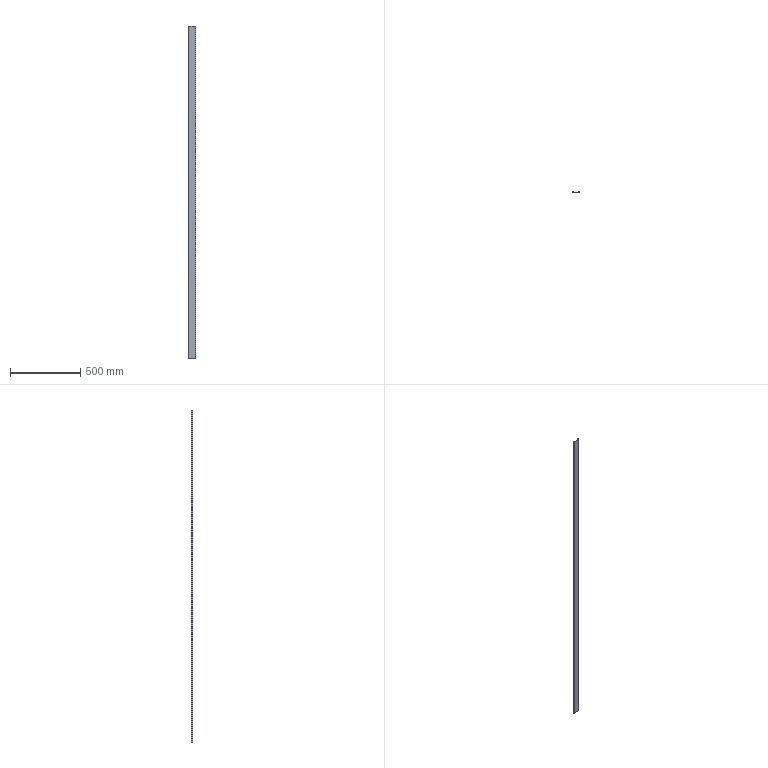Part | STEP file | 31E-01026QY25 | 1 solid | 32 faces | box 50 x 9.195 x 2366 mm | volume 207531 mm3 | cylinder 16 | plane 16 | commonest cylinder face diameters 1 x8 1.2 x6 2 x2
STEP:
#1=CARTESIAN_POINT('',(0.2485,8.595,1183.));
#2=VERTEX_POINT('',#1);
#3=CARTESIAN_POINT('',(0.4243,8.171,1183.));
#4=VERTEX_POINT('',#3);
#5=CARTESIAN_POINT('',(0.8485,8.595,1183.));
#6=DIRECTION('',(0.,0.,-1.));
#7=AXIS2_PLACEMENT_3D('',#5,#6,$);
#8=CIRCLE('',#7,0.6);
#9=EDGE_CURVE('',#2,#4,#8,.F.);
#10=ORIENTED_EDGE('',*,*,#9,.F.);
#11=CARTESIAN_POINT('',(0.2485,8.595,-1183.));
#12=VERTEX_POINT('',#11);
#13=CARTESIAN_POINT('',(0.2485,8.595,1183.));
#14=DIRECTION('',(0.,0.,-1.));
#15=VECTOR('',#14,1.);
#16=LINE('',#13,#15);
#17=EDGE_CURVE('',#2,#12,#16,.T.);
#18=ORIENTED_EDGE('',*,*,#17,.T.);
#19=CARTESIAN_POINT('',(0.4243,8.171,-1183.));
#20=VERTEX_POINT('',#19);
#21=CARTESIAN_POINT('',(0.8485,8.595,-1183.));
#22=DIRECTION('',(0.,0.,-1.));
#23=AXIS2_PLACEMENT_3D('',#21,#22,$);
#24=CIRCLE('',#23,0.6);
#25=EDGE_CURVE('',#20,#12,#24,.T.);
#26=ORIENTED_EDGE('',*,*,#25,.F.);
#27=CARTESIAN_POINT('',(0.4243,8.171,1183.));
#28=DIRECTION('',(0.,0.,-1.));
#29=VECTOR('',#28,1.);
#30=LINE('',#27,#29);
#31=EDGE_CURVE('',#4,#20,#30,.T.);
#32=ORIENTED_EDGE('',*,*,#31,.F.);
#33=EDGE_LOOP('',(#10,#18,#26,#32));
#34=FACE_OUTER_BOUND('',#33,.T.);
#35=CARTESIAN_POINT('',(0.8485,8.595,1183.));
#36=DIRECTION('',(0.,0.,-1.));
#37=DIRECTION('',(1.,0.,0.));
#38=AXIS2_PLACEMENT_3D('',#35,#36,#37);
#39=CYLINDRICAL_SURFACE('',#38,0.6);
#40=ADVANCED_FACE('',(#34),#39,.T.);
#41=CARTESIAN_POINT('',(1.273,9.019,1183.));
#42=VERTEX_POINT('',#41);
#43=CARTESIAN_POINT('',(0.4243,9.019,1183.));
#44=VERTEX_POINT('',#43);
#45=CARTESIAN_POINT('',(1.273,9.019,1183.));
#46=CARTESIAN_POINT('',(1.219,9.073,1183.));
#47=CARTESIAN_POINT('',(1.158,9.118,1183.));
#48=CARTESIAN_POINT('',(1.089,9.152,1183.));
#49=CARTESIAN_POINT('',(0.9442,9.199,1183.));
#50=CARTESIAN_POINT('',(0.7916,9.2,1183.));
#51=CARTESIAN_POINT('',(0.7159,9.188,1183.));
#52=CARTESIAN_POINT('',(0.6071,9.152,1183.));
#53=CARTESIAN_POINT('',(0.5104,9.093,1183.));
#54=CARTESIAN_POINT('',(0.4796,9.07,1183.));
#55=CARTESIAN_POINT('',(0.4509,9.046,1183.));
#56=CARTESIAN_POINT('',(0.4243,9.019,1183.));
#57=B_SPLINE_CURVE_WITH_KNOTS('',5,(#45,#46,#47,#48,#49,#50,#51,#52,#53,#54,#55,#56),.UNSPECIFIED.,.F.,.U.,(6,3,3,6),(0.,0.5331,1.066,1.332),.UNSPECIFIED.);
#58=EDGE_CURVE('',#42,#44,#57,.T.);
#59=ORIENTED_EDGE('',*,*,#58,.T.);
#60=CARTESIAN_POINT('',(0.4243,9.019,1183.));
#61=CARTESIAN_POINT('',(0.3843,8.979,1183.));
#62=CARTESIAN_POINT('',(0.349,8.935,1183.));
#63=CARTESIAN_POINT('',(0.3192,8.886,1183.));
#64=CARTESIAN_POINT('',(0.2795,8.8,1183.));
#65=CARTESIAN_POINT('',(0.2574,8.708,1183.));
#66=CARTESIAN_POINT('',(0.2515,8.67,1183.));
#67=CARTESIAN_POINT('',(0.2485,8.633,1183.));
#68=CARTESIAN_POINT('',(0.2485,8.595,1183.));
#69=B_SPLINE_CURVE_WITH_KNOTS('',5,(#60,#61,#62,#63,#64,#65,#66,#67,#68),.UNSPECIFIED.,.F.,.U.,(6,3,6),(0.,0.3999,0.6659),.UNSPECIFIED.);
#70=EDGE_CURVE('',#44,#2,#69,.T.);
#71=ORIENTED_EDGE('',*,*,#70,.T.);
#72=ORIENTED_EDGE('',*,*,#9,.T.);
#73=CARTESIAN_POINT('',(2.898,5.697,1183.));
#74=VERTEX_POINT('',#73);
#75=CARTESIAN_POINT('',(1.661,6.934,1183.));
#76=DIRECTION('',(0.7071,-0.7071,0.));
#77=VECTOR('',#76,1.);
#78=LINE('',#75,#77);
#79=EDGE_CURVE('',#4,#74,#78,.T.);
#80=ORIENTED_EDGE('',*,*,#79,.T.);
#81=CARTESIAN_POINT('',(0.3706,5.02,1183.));
#82=VERTEX_POINT('',#81);
#83=CARTESIAN_POINT('',(1.634,5.359,1183.));
#84=DIRECTION('',(-0.9659,-0.2588,0.));
#85=VECTOR('',#84,1.);
#86=LINE('',#83,#85);
#87=EDGE_CURVE('',#74,#82,#86,.T.);
#88=ORIENTED_EDGE('',*,*,#87,.T.);
#89=CARTESIAN_POINT('',(0.,4.537,1183.));
#90=VERTEX_POINT('',#89);
#91=CARTESIAN_POINT('',(0.3706,5.02,1183.));
#92=CARTESIAN_POINT('',(0.32,5.007,1183.));
#93=CARTESIAN_POINT('',(0.2712,4.986,1183.));
#94=CARTESIAN_POINT('',(0.2253,4.96,1183.));
#95=CARTESIAN_POINT('',(0.1416,4.896,1183.));
#96=CARTESIAN_POINT('',(0.07725,4.812,1183.));
#97=CARTESIAN_POINT('',(0.05076,4.766,1183.));
#98=CARTESIAN_POINT('',(0.02052,4.693,1183.));
#99=CARTESIAN_POINT('',(0.005155,4.616,1183.));
#100=CARTESIAN_POINT('',(0.001709,4.589,1183.));
#101=CARTESIAN_POINT('',(0.,4.563,1183.));
#102=CARTESIAN_POINT('',(0.,4.537,1183.));
#103=B_SPLINE_CURVE_WITH_KNOTS('',5,(#91,#92,#93,#94,#95,#96,#97,#98,#99,#100,#101,#102),.UNSPECIFIED.,.F.,.U.,(6,3,3,6),(0.,0.3702,0.7405,0.9253),.UNSPECIFIED.);
#104=EDGE_CURVE('',#82,#90,#103,.T.);
#105=ORIENTED_EDGE('',*,*,#104,.T.);
#106=CARTESIAN_POINT('',(0.,1.,1183.));
#107=VERTEX_POINT('',#106);
#108=CARTESIAN_POINT('',(0.,2.769,1183.));
#109=DIRECTION('',(0.,-1.,0.));
#110=VECTOR('',#109,1.);
#111=LINE('',#108,#110);
#112=EDGE_CURVE('',#90,#107,#111,.T.);
#113=ORIENTED_EDGE('',*,*,#112,.T.);
#114=CARTESIAN_POINT('',(1.,0.,1183.));
#115=VERTEX_POINT('',#114);
#116=CARTESIAN_POINT('',(0.,1.,1183.));
#117=CARTESIAN_POINT('',(0.,0.902,1183.));
#118=CARTESIAN_POINT('',(0.012,0.804,1183.));
#119=CARTESIAN_POINT('',(0.036,0.708,1183.));
#120=CARTESIAN_POINT('',(0.107,0.5238,1183.));
#121=CARTESIAN_POINT('',(0.2204,0.3622,1183.));
#122=CARTESIAN_POINT('',(0.2868,0.2888,1183.));
#123=CARTESIAN_POINT('',(0.4361,0.1597,1183.));
#124=CARTESIAN_POINT('',(0.6122,0.0704,1183.));
#125=CARTESIAN_POINT('',(0.7053,0.03682,1183.));
#126=CARTESIAN_POINT('',(0.8215,0.01049,1183.));
#127=CARTESIAN_POINT('',(0.9393,0.001534,1183.));
#128=CARTESIAN_POINT('',(0.9596,0.0005109,1183.));
#129=CARTESIAN_POINT('',(0.9798,0.000000001,1183.));
#130=CARTESIAN_POINT('',(1.,0.000000001,1183.));
#131=B_SPLINE_CURVE_WITH_KNOTS('',5,(#116,#117,#118,#119,#120,#121,#122,#123,#124,#125,#126,#127,#128,#129,#130),.UNSPECIFIED.,.F.,.U.,(6,3,3,3,6),(0.,0.6928,1.386,2.078,2.221),.UNSPECIFIED.);
#132=EDGE_CURVE('',#107,#115,#131,.T.);
#133=ORIENTED_EDGE('',*,*,#132,.T.);
#134=CARTESIAN_POINT('',(49.,0.,1183.));
#135=VERTEX_POINT('',#134);
#136=CARTESIAN_POINT('',(25.,0.000000001,1183.));
#137=DIRECTION('',(1.,0.,0.));
#138=VECTOR('',#137,1.);
#139=LINE('',#136,#138);
#140=EDGE_CURVE('',#115,#135,#139,.T.);
#141=ORIENTED_EDGE('',*,*,#140,.T.);
#142=CARTESIAN_POINT('',(50.,1.,1183.));
#143=VERTEX_POINT('',#142);
#144=CARTESIAN_POINT('',(49.,0.000000001,1183.));
#145=CARTESIAN_POINT('',(49.098,0.000000001,1183.));
#146=CARTESIAN_POINT('',(49.196,0.012,1183.));
#147=CARTESIAN_POINT('',(49.292,0.036,1183.));
#148=CARTESIAN_POINT('',(49.476,0.107,1183.));
#149=CARTESIAN_POINT('',(49.638,0.2204,1183.));
#150=CARTESIAN_POINT('',(49.711,0.2868,1183.));
#151=CARTESIAN_POINT('',(49.84,0.4361,1183.));
#152=CARTESIAN_POINT('',(49.93,0.6122,1183.));
#153=CARTESIAN_POINT('',(49.963,0.7053,1183.));
#154=CARTESIAN_POINT('',(49.99,0.8215,1183.));
#155=CARTESIAN_POINT('',(49.998,0.9393,1183.));
#156=CARTESIAN_POINT('',(49.999,0.9596,1183.));
#157=CARTESIAN_POINT('',(50.,0.9798,1183.));
#158=CARTESIAN_POINT('',(50.,1.,1183.));
#159=B_SPLINE_CURVE_WITH_KNOTS('',5,(#144,#145,#146,#147,#148,#149,#150,#151,#152,#153,#154,#155,#156,#157,#158),.UNSPECIFIED.,.F.,.U.,(6,3,3,3,6),(0.,0.6928,1.386,2.078,2.221),.UNSPECIFIED.);
#160=EDGE_CURVE('',#135,#143,#159,.T.);
#161=ORIENTED_EDGE('',*,*,#160,.T.);
#162=CARTESIAN_POINT('',(50.,4.537,1183.));
#163=VERTEX_POINT('',#162);
#164=CARTESIAN_POINT('',(50.,2.769,1183.));
#165=DIRECTION('',(0.,1.,0.));
#166=VECTOR('',#165,1.);
#167=LINE('',#164,#166);
#168=EDGE_CURVE('',#143,#163,#167,.T.);
#169=ORIENTED_EDGE('',*,*,#168,.T.);
#170=CARTESIAN_POINT('',(49.629,5.02,1183.));
#171=VERTEX_POINT('',#170);
#172=CARTESIAN_POINT('',(50.,4.537,1183.));
#173=CARTESIAN_POINT('',(50.,4.589,1183.));
#174=CARTESIAN_POINT('',(49.993,4.642,1183.));
#175=CARTESIAN_POINT('',(49.979,4.693,1183.));
#176=CARTESIAN_POINT('',(49.939,4.791,1183.));
#177=CARTESIAN_POINT('',(49.875,4.874,1183.));
#178=CARTESIAN_POINT('',(49.837,4.912,1183.));
#179=CARTESIAN_POINT('',(49.774,4.96,1183.));
#180=CARTESIAN_POINT('',(49.704,4.995,1183.));
#181=CARTESIAN_POINT('',(49.679,5.005,1183.));
#182=CARTESIAN_POINT('',(49.655,5.013,1183.));
#183=CARTESIAN_POINT('',(49.629,5.02,1183.));
#184=B_SPLINE_CURVE_WITH_KNOTS('',5,(#172,#173,#174,#175,#176,#177,#178,#179,#180,#181,#182,#183),.UNSPECIFIED.,.F.,.U.,(6,3,3,6),(0.,0.3702,0.7405,0.9253),.UNSPECIFIED.);
#185=EDGE_CURVE('',#163,#171,#184,.T.);
#186=ORIENTED_EDGE('',*,*,#185,.T.);
#187=CARTESIAN_POINT('',(47.102,5.697,1183.));
#188=VERTEX_POINT('',#187);
#189=CARTESIAN_POINT('',(48.366,5.359,1183.));
#190=DIRECTION('',(-0.9659,0.2588,0.));
#191=VECTOR('',#190,1.);
#192=LINE('',#189,#191);
#193=EDGE_CURVE('',#171,#188,#192,.T.);
#194=ORIENTED_EDGE('',*,*,#193,.T.);
#195=CARTESIAN_POINT('',(49.576,8.171,1183.));
#196=VERTEX_POINT('',#195);
#197=CARTESIAN_POINT('',(48.339,6.934,1183.));
#198=DIRECTION('',(0.7071,0.7071,0.));
#199=VECTOR('',#198,1.);
#200=LINE('',#197,#199);
#201=EDGE_CURVE('',#188,#196,#200,.T.);
#202=ORIENTED_EDGE('',*,*,#201,.T.);
#203=CARTESIAN_POINT('',(49.751,8.595,1183.));
#204=VERTEX_POINT('',#203);
#205=CARTESIAN_POINT('',(49.576,8.171,1183.));
#206=CARTESIAN_POINT('',(49.629,8.224,1183.));
#207=CARTESIAN_POINT('',(49.674,8.286,1183.));
#208=CARTESIAN_POINT('',(49.709,8.354,1183.));
#209=CARTESIAN_POINT('',(49.738,8.445,1183.));
#210=CARTESIAN_POINT('',(49.749,8.539,1183.));
#211=CARTESIAN_POINT('',(49.751,8.557,1183.));
#212=CARTESIAN_POINT('',(49.751,8.576,1183.));
#213=CARTESIAN_POINT('',(49.751,8.595,1183.));
#214=B_SPLINE_CURVE_WITH_KNOTS('',5,(#205,#206,#207,#208,#209,#210,#211,#212,#213),.UNSPECIFIED.,.F.,.U.,(6,3,6),(0.,0.5331,0.6664),.UNSPECIFIED.);
#215=EDGE_CURVE('',#196,#204,#214,.T.);
#216=ORIENTED_EDGE('',*,*,#215,.T.);
#217=CARTESIAN_POINT('',(49.576,9.019,1183.));
#218=VERTEX_POINT('',#217);
#219=CARTESIAN_POINT('',(49.751,8.595,1183.));
#220=CARTESIAN_POINT('',(49.751,8.652,1183.));
#221=CARTESIAN_POINT('',(49.745,8.708,1183.));
#222=CARTESIAN_POINT('',(49.731,8.764,1183.));
#223=CARTESIAN_POINT('',(49.699,8.853,1183.));
#224=CARTESIAN_POINT('',(49.649,8.933,1183.));
#225=CARTESIAN_POINT('',(49.627,8.964,1183.));
#226=CARTESIAN_POINT('',(49.602,8.993,1183.));
#227=CARTESIAN_POINT('',(49.576,9.019,1183.));
#228=B_SPLINE_CURVE_WITH_KNOTS('',5,(#219,#220,#221,#222,#223,#224,#225,#226,#227),.UNSPECIFIED.,.F.,.U.,(6,3,6),(0.6664,1.066,1.332),.UNSPECIFIED.);
#229=EDGE_CURVE('',#204,#218,#228,.T.);
#230=ORIENTED_EDGE('',*,*,#229,.T.);
#231=CARTESIAN_POINT('',(48.727,9.019,1183.));
#232=VERTEX_POINT('',#231);
#233=CARTESIAN_POINT('',(49.576,9.019,1183.));
#234=CARTESIAN_POINT('',(49.522,9.073,1183.));
#235=CARTESIAN_POINT('',(49.461,9.118,1183.));
#236=CARTESIAN_POINT('',(49.392,9.152,1183.));
#237=CARTESIAN_POINT('',(49.247,9.199,1183.));
#238=CARTESIAN_POINT('',(49.095,9.2,1183.));
#239=CARTESIAN_POINT('',(49.019,9.188,1183.));
#240=CARTESIAN_POINT('',(48.91,9.152,1183.));
#241=CARTESIAN_POINT('',(48.813,9.093,1183.));
#242=CARTESIAN_POINT('',(48.782,9.07,1183.));
#243=CARTESIAN_POINT('',(48.754,9.046,1183.));
#244=CARTESIAN_POINT('',(48.727,9.019,1183.));
#245=B_SPLINE_CURVE_WITH_KNOTS('',5,(#233,#234,#235,#236,#237,#238,#239,#240,#241,#242,#243,#244),.UNSPECIFIED.,.F.,.U.,(6,3,3,6),(0.,0.5331,1.066,1.332),.UNSPECIFIED.);
#246=EDGE_CURVE('',#218,#232,#245,.T.);
#247=ORIENTED_EDGE('',*,*,#246,.T.);
#248=CARTESIAN_POINT('',(45.396,5.688,1183.));
#249=VERTEX_POINT('',#248);
#250=CARTESIAN_POINT('',(47.062,7.354,1183.));
#251=DIRECTION('',(-0.7071,-0.7071,0.));
#252=VECTOR('',#251,1.);
#253=LINE('',#250,#252);
#254=EDGE_CURVE('',#232,#249,#253,.T.);
#255=ORIENTED_EDGE('',*,*,#254,.T.);
#256=CARTESIAN_POINT('',(45.25,5.335,1183.));
#257=VERTEX_POINT('',#256);
#258=CARTESIAN_POINT('',(45.396,5.688,1183.));
#259=CARTESIAN_POINT('',(45.363,5.655,1183.));
#260=CARTESIAN_POINT('',(45.334,5.618,1183.));
#261=CARTESIAN_POINT('',(45.309,5.577,1183.));
#262=CARTESIAN_POINT('',(45.276,5.506,1183.));
#263=CARTESIAN_POINT('',(45.257,5.429,1183.));
#264=CARTESIAN_POINT('',(45.252,5.398,1183.));
#265=CARTESIAN_POINT('',(45.25,5.366,1183.));
#266=CARTESIAN_POINT('',(45.25,5.335,1183.));
#267=B_SPLINE_CURVE_WITH_KNOTS('',5,(#258,#259,#260,#261,#262,#263,#264,#265,#266),.UNSPECIFIED.,.F.,.U.,(6,3,6),(0.,0.3332,0.5549),.UNSPECIFIED.);
#268=EDGE_CURVE('',#249,#257,#267,.T.);
#269=ORIENTED_EDGE('',*,*,#268,.T.);
#270=CARTESIAN_POINT('',(45.621,4.852,1183.));
#271=VERTEX_POINT('',#270);
#272=CARTESIAN_POINT('',(45.25,5.335,1183.));
#273=CARTESIAN_POINT('',(45.25,5.283,1183.));
#274=CARTESIAN_POINT('',(45.257,5.23,1183.));
#275=CARTESIAN_POINT('',(45.27,5.179,1183.));
#276=CARTESIAN_POINT('',(45.311,5.081,1183.));
#277=CARTESIAN_POINT('',(45.375,4.998,1183.));
#278=CARTESIAN_POINT('',(45.413,4.96,1183.));
#279=CARTESIAN_POINT('',(45.476,4.912,1183.));
#280=CARTESIAN_POINT('',(45.546,4.877,1183.));
#281=CARTESIAN_POINT('',(45.57,4.867,1183.));
#282=CARTESIAN_POINT('',(45.595,4.859,1183.));
#283=CARTESIAN_POINT('',(45.621,4.852,1183.));
#284=B_SPLINE_CURVE_WITH_KNOTS('',5,(#272,#273,#274,#275,#276,#277,#278,#279,#280,#281,#282,#283),.UNSPECIFIED.,.F.,.U.,(6,3,3,6),(0.,0.3702,0.7405,0.9253),.UNSPECIFIED.);
#285=EDGE_CURVE('',#257,#271,#284,.T.);
#286=ORIENTED_EDGE('',*,*,#285,.T.);
#287=CARTESIAN_POINT('',(48.8,4.,1183.));
#288=VERTEX_POINT('',#287);
#289=CARTESIAN_POINT('',(47.21,4.426,1183.));
#290=DIRECTION('',(0.9659,-0.2588,0.));
#291=VECTOR('',#290,1.);
#292=LINE('',#289,#291);
#293=EDGE_CURVE('',#271,#288,#292,.T.);
#294=ORIENTED_EDGE('',*,*,#293,.T.);
#295=CARTESIAN_POINT('',(48.8,1.7,1183.));
#296=VERTEX_POINT('',#295);
#297=CARTESIAN_POINT('',(48.8,2.85,1183.));
#298=DIRECTION('',(0.,-1.,0.));
#299=VECTOR('',#298,1.);
#300=LINE('',#297,#299);
#301=EDGE_CURVE('',#288,#296,#300,.T.);
#302=ORIENTED_EDGE('',*,*,#301,.T.);
#303=CARTESIAN_POINT('',(48.3,1.2,1183.));
#304=VERTEX_POINT('',#303);
#305=CARTESIAN_POINT('',(48.3,1.7,1183.));
#306=DIRECTION('',(0.,0.,-1.));
#307=AXIS2_PLACEMENT_3D('',#305,#306,$);
#308=CIRCLE('',#307,0.5);
#309=EDGE_CURVE('',#296,#304,#308,.T.);
#310=ORIENTED_EDGE('',*,*,#309,.T.);
#311=CARTESIAN_POINT('',(1.7,1.2,1183.));
#312=VERTEX_POINT('',#311);
#313=CARTESIAN_POINT('',(25.,1.2,1183.));
#314=DIRECTION('',(-1.,0.,0.));
#315=VECTOR('',#314,1.);
#316=LINE('',#313,#315);
#317=EDGE_CURVE('',#304,#312,#316,.T.);
#318=ORIENTED_EDGE('',*,*,#317,.T.);
#319=CARTESIAN_POINT('',(1.2,1.7,1183.));
#320=VERTEX_POINT('',#319);
#321=CARTESIAN_POINT('',(1.7,1.7,1183.));
#322=DIRECTION('',(0.,0.,-1.));
#323=AXIS2_PLACEMENT_3D('',#321,#322,$);
#324=CIRCLE('',#323,0.5);
#325=EDGE_CURVE('',#312,#320,#324,.T.);
#326=ORIENTED_EDGE('',*,*,#325,.T.);
#327=CARTESIAN_POINT('',(1.2,4.,1183.));
#328=VERTEX_POINT('',#327);
#329=CARTESIAN_POINT('',(1.2,2.85,1183.));
#330=DIRECTION('',(0.,1.,0.));
#331=VECTOR('',#330,1.);
#332=LINE('',#329,#331);
#333=EDGE_CURVE('',#320,#328,#332,.T.);
#334=ORIENTED_EDGE('',*,*,#333,.T.);
#335=CARTESIAN_POINT('',(4.379,4.852,1183.));
#336=VERTEX_POINT('',#335);
#337=CARTESIAN_POINT('',(2.79,4.426,1183.));
#338=DIRECTION('',(0.9659,0.2588,0.));
#339=VECTOR('',#338,1.);
#340=LINE('',#337,#339);
#341=EDGE_CURVE('',#328,#336,#340,.T.);
#342=ORIENTED_EDGE('',*,*,#341,.T.);
#343=CARTESIAN_POINT('',(4.75,5.335,1183.));
#344=VERTEX_POINT('',#343);
#345=CARTESIAN_POINT('',(4.379,4.852,1183.));
#346=CARTESIAN_POINT('',(4.446,4.87,1183.));
#347=CARTESIAN_POINT('',(4.51,4.899,1183.));
#348=CARTESIAN_POINT('',(4.568,4.94,1183.));
#349=CARTESIAN_POINT('',(4.662,5.034,1183.));
#350=CARTESIAN_POINT('',(4.722,5.152,1183.));
#351=CARTESIAN_POINT('',(4.741,5.212,1183.));
#352=CARTESIAN_POINT('',(4.75,5.273,1183.));
#353=CARTESIAN_POINT('',(4.75,5.335,1183.));
#354=B_SPLINE_CURVE_WITH_KNOTS('',5,(#345,#346,#347,#348,#349,#350,#351,#352,#353),.UNSPECIFIED.,.F.,.U.,(6,3,6),(0.,0.4899,0.9256),.UNSPECIFIED.);
#355=EDGE_CURVE('',#336,#344,#354,.T.);
#356=ORIENTED_EDGE('',*,*,#355,.T.);
#357=CARTESIAN_POINT('',(4.604,5.688,1183.));
#358=VERTEX_POINT('',#357);
#359=CARTESIAN_POINT('',(4.75,5.335,1183.));
#360=CARTESIAN_POINT('',(4.75,5.343,1183.));
#361=CARTESIAN_POINT('',(4.75,5.35,1183.));
#362=CARTESIAN_POINT('',(4.75,5.358,1183.));
#363=CARTESIAN_POINT('',(4.745,5.435,1183.));
#364=CARTESIAN_POINT('',(4.726,5.51,1183.));
#365=CARTESIAN_POINT('',(4.697,5.575,1183.));
#366=CARTESIAN_POINT('',(4.657,5.634,1183.));
#367=CARTESIAN_POINT('',(4.607,5.685,1183.));
#368=CARTESIAN_POINT('',(4.606,5.686,1183.));
#369=CARTESIAN_POINT('',(4.605,5.687,1183.));
#370=CARTESIAN_POINT('',(4.604,5.688,1183.));
#371=B_SPLINE_CURVE_WITH_KNOTS('',5,(#359,#360,#361,#362,#363,#364,#365,#366,#367,#368,#369,#370),.UNSPECIFIED.,.F.,.U.,(6,3,3,6),(0.9256,0.9798,1.47,1.481),.UNSPECIFIED.);
#372=EDGE_CURVE('',#344,#358,#371,.T.);
#373=ORIENTED_EDGE('',*,*,#372,.T.);
#374=CARTESIAN_POINT('',(2.938,7.354,1183.));
#375=DIRECTION('',(-0.7071,0.7071,0.));
#376=VECTOR('',#375,1.);
#377=LINE('',#374,#376);
#378=EDGE_CURVE('',#358,#42,#377,.T.);
#379=ORIENTED_EDGE('',*,*,#378,.T.);
#380=EDGE_LOOP('',(#59,#71,#72,#80,#88,#105,#113,#133,#141,#161,#169,#186,#194,#202,#216,#230,#247,#255,#269,#286,#294,#302,#310,#318,#326,#334,#342,#356,#373,#379));
#381=FACE_OUTER_BOUND('',#380,.T.);
#382=CARTESIAN_POINT('',(0.,1.2,1183.));
#383=DIRECTION('',(0.,0.,-1.));
#384=DIRECTION('',(-1.,0.,0.));
#385=AXIS2_PLACEMENT_3D('',#382,#383,#384);
#386=PLANE('',#385);
#387=ADVANCED_FACE('',(#381),#386,.F.);
#388=ORIENTED_EDGE('',*,*,#17,.F.);
#389=ORIENTED_EDGE('',*,*,#70,.F.);
#390=CARTESIAN_POINT('',(0.4243,9.019,-1183.));
#391=VERTEX_POINT('',#390);
#392=CARTESIAN_POINT('',(0.4243,9.019,1183.));
#393=DIRECTION('',(0.,0.,-1.));
#394=VECTOR('',#393,1.);
#395=LINE('',#392,#394);
#396=EDGE_CURVE('',#44,#391,#395,.T.);
#397=ORIENTED_EDGE('',*,*,#396,.T.);
#398=CARTESIAN_POINT('',(0.8485,8.595,-1183.));
#399=DIRECTION('',(0.,0.,-1.));
#400=AXIS2_PLACEMENT_3D('',#398,#399,$);
#401=CIRCLE('',#400,0.6);
#402=EDGE_CURVE('',#12,#391,#401,.T.);
#403=ORIENTED_EDGE('',*,*,#402,.F.);
#404=EDGE_LOOP('',(#388,#389,#397,#403));
#405=FACE_OUTER_BOUND('',#404,.T.);
#406=CARTESIAN_POINT('',(0.8485,8.595,1183.));
#407=DIRECTION('',(0.,0.,-1.));
#408=DIRECTION('',(-1.,0.,0.));
#409=AXIS2_PLACEMENT_3D('',#406,#407,#408);
#410=CYLINDRICAL_SURFACE('',#409,0.6);
#411=ADVANCED_FACE('',(#405),#410,.T.);
#412=CARTESIAN_POINT('',(2.898,5.697,-1183.));
#413=VERTEX_POINT('',#412);
#414=CARTESIAN_POINT('',(1.661,6.934,-1183.));
#415=DIRECTION('',(0.7071,-0.7071,0.));
#416=VECTOR('',#415,1.);
#417=LINE('',#414,#416);
#418=EDGE_CURVE('',#20,#413,#417,.T.);
#419=ORIENTED_EDGE('',*,*,#418,.F.);
#420=ORIENTED_EDGE('',*,*,#25,.T.);
#421=ORIENTED_EDGE('',*,*,#402,.T.);
#422=CARTESIAN_POINT('',(1.273,9.019,-1183.));
#423=VERTEX_POINT('',#422);
#424=CARTESIAN_POINT('',(0.8485,8.595,-1183.));
#425=DIRECTION('',(0.,0.,-1.));
#426=AXIS2_PLACEMENT_3D('',#424,#425,$);
#427=CIRCLE('',#426,0.6);
#428=EDGE_CURVE('',#391,#423,#427,.T.);
#429=ORIENTED_EDGE('',*,*,#428,.T.);
#430=CARTESIAN_POINT('',(4.604,5.688,-1183.));
#431=VERTEX_POINT('',#430);
#432=CARTESIAN_POINT('',(2.938,7.354,-1183.));
#433=DIRECTION('',(-0.7071,0.7071,0.));
#434=VECTOR('',#433,1.);
#435=LINE('',#432,#434);
#436=EDGE_CURVE('',#431,#423,#435,.T.);
#437=ORIENTED_EDGE('',*,*,#436,.F.);
#438=CARTESIAN_POINT('',(4.75,5.335,-1183.));
#439=VERTEX_POINT('',#438);
#440=CARTESIAN_POINT('',(4.25,5.335,-1183.));
#441=DIRECTION('',(0.,0.,-1.));
#442=AXIS2_PLACEMENT_3D('',#440,#441,$);
#443=CIRCLE('',#442,0.5);
#444=EDGE_CURVE('',#431,#439,#443,.T.);
#445=ORIENTED_EDGE('',*,*,#444,.T.);
#446=CARTESIAN_POINT('',(4.379,4.852,-1183.));
#447=VERTEX_POINT('',#446);
#448=CARTESIAN_POINT('',(4.25,5.335,-1183.));
#449=DIRECTION('',(0.,0.,-1.));
#450=AXIS2_PLACEMENT_3D('',#448,#449,$);
#451=CIRCLE('',#450,0.5);
#452=EDGE_CURVE('',#439,#447,#451,.T.);
#453=ORIENTED_EDGE('',*,*,#452,.T.);
#454=CARTESIAN_POINT('',(1.2,4.,-1183.));
#455=VERTEX_POINT('',#454);
#456=CARTESIAN_POINT('',(2.79,4.426,-1183.));
#457=DIRECTION('',(0.9659,0.2588,0.));
#458=VECTOR('',#457,1.);
#459=LINE('',#456,#458);
#460=EDGE_CURVE('',#455,#447,#459,.T.);
#461=ORIENTED_EDGE('',*,*,#460,.F.);
#462=CARTESIAN_POINT('',(1.2,1.7,-1183.));
#463=VERTEX_POINT('',#462);
#464=CARTESIAN_POINT('',(1.2,2.85,-1183.));
#465=DIRECTION('',(0.,1.,0.));
#466=VECTOR('',#465,1.);
#467=LINE('',#464,#466);
#468=EDGE_CURVE('',#463,#455,#467,.T.);
#469=ORIENTED_EDGE('',*,*,#468,.F.);
#470=CARTESIAN_POINT('',(1.7,1.2,-1183.));
#471=VERTEX_POINT('',#470);
#472=CARTESIAN_POINT('',(1.2,1.7,-1183.));
#473=CARTESIAN_POINT('',(1.2,1.637,-1183.));
#474=CARTESIAN_POINT('',(1.21,1.574,-1183.));
#475=CARTESIAN_POINT('',(1.23,1.514,-1183.));
#476=CARTESIAN_POINT('',(1.288,1.4,-1183.));
#477=CARTESIAN_POINT('',(1.377,1.31,-1183.));
#478=CARTESIAN_POINT('',(1.429,1.273,-1183.));
#479=CARTESIAN_POINT('',(1.514,1.23,-1183.));
#480=CARTESIAN_POINT('',(1.606,1.207,-1183.));
#481=CARTESIAN_POINT('',(1.637,1.202,-1183.));
#482=CARTESIAN_POINT('',(1.669,1.2,-1183.));
#483=CARTESIAN_POINT('',(1.7,1.2,-1183.));
#484=B_SPLINE_CURVE_WITH_KNOTS('',5,(#472,#473,#474,#475,#476,#477,#478,#479,#480,#481,#482,#483),.UNSPECIFIED.,.F.,.U.,(6,3,3,6),(0.,0.4443,0.8886,1.11),.UNSPECIFIED.);
#485=EDGE_CURVE('',#463,#471,#484,.T.);
#486=ORIENTED_EDGE('',*,*,#485,.T.);
#487=CARTESIAN_POINT('',(48.3,1.2,-1183.));
#488=VERTEX_POINT('',#487);
#489=CARTESIAN_POINT('',(25.,1.2,-1183.));
#490=DIRECTION('',(-1.,0.,0.));
#491=VECTOR('',#490,1.);
#492=LINE('',#489,#491);
#493=EDGE_CURVE('',#488,#471,#492,.T.);
#494=ORIENTED_EDGE('',*,*,#493,.F.);
#495=CARTESIAN_POINT('',(48.8,1.7,-1183.));
#496=VERTEX_POINT('',#495);
#497=CARTESIAN_POINT('',(48.3,1.2,-1183.));
#498=CARTESIAN_POINT('',(48.363,1.2,-1183.));
#499=CARTESIAN_POINT('',(48.426,1.21,-1183.));
#500=CARTESIAN_POINT('',(48.486,1.23,-1183.));
#501=CARTESIAN_POINT('',(48.6,1.288,-1183.));
#502=CARTESIAN_POINT('',(48.69,1.377,-1183.));
#503=CARTESIAN_POINT('',(48.727,1.429,-1183.));
#504=CARTESIAN_POINT('',(48.77,1.514,-1183.));
#505=CARTESIAN_POINT('',(48.793,1.606,-1183.));
#506=CARTESIAN_POINT('',(48.798,1.637,-1183.));
#507=CARTESIAN_POINT('',(48.8,1.669,-1183.));
#508=CARTESIAN_POINT('',(48.8,1.7,-1183.));
#509=B_SPLINE_CURVE_WITH_KNOTS('',5,(#497,#498,#499,#500,#501,#502,#503,#504,#505,#506,#507,#508),.UNSPECIFIED.,.F.,.U.,(6,3,3,6),(0.,0.4443,0.8886,1.11),.UNSPECIFIED.);
#510=EDGE_CURVE('',#488,#496,#509,.T.);
#511=ORIENTED_EDGE('',*,*,#510,.T.);
#512=CARTESIAN_POINT('',(48.8,4.,-1183.));
#513=VERTEX_POINT('',#512);
#514=CARTESIAN_POINT('',(48.8,2.85,-1183.));
#515=DIRECTION('',(0.,-1.,0.));
#516=VECTOR('',#515,1.);
#517=LINE('',#514,#516);
#518=EDGE_CURVE('',#513,#496,#517,.T.);
#519=ORIENTED_EDGE('',*,*,#518,.F.);
#520=CARTESIAN_POINT('',(45.621,4.852,-1183.));
#521=VERTEX_POINT('',#520);
#522=CARTESIAN_POINT('',(47.21,4.426,-1183.));
#523=DIRECTION('',(0.9659,-0.2588,0.));
#524=VECTOR('',#523,1.);
#525=LINE('',#522,#524);
#526=EDGE_CURVE('',#521,#513,#525,.T.);
#527=ORIENTED_EDGE('',*,*,#526,.F.);
#528=CARTESIAN_POINT('',(45.25,5.335,-1183.));
#529=VERTEX_POINT('',#528);
#530=CARTESIAN_POINT('',(45.75,5.335,-1183.));
#531=DIRECTION('',(0.,0.,-1.));
#532=AXIS2_PLACEMENT_3D('',#530,#531,$);
#533=CIRCLE('',#532,0.5);
#534=EDGE_CURVE('',#521,#529,#533,.T.);
#535=ORIENTED_EDGE('',*,*,#534,.T.);
#536=CARTESIAN_POINT('',(45.396,5.688,-1183.));
#537=VERTEX_POINT('',#536);
#538=CARTESIAN_POINT('',(45.75,5.335,-1183.));
#539=DIRECTION('',(0.,0.,-1.));
#540=AXIS2_PLACEMENT_3D('',#538,#539,$);
#541=CIRCLE('',#540,0.5);
#542=EDGE_CURVE('',#529,#537,#541,.T.);
#543=ORIENTED_EDGE('',*,*,#542,.T.);
#544=CARTESIAN_POINT('',(48.727,9.019,-1183.));
#545=VERTEX_POINT('',#544);
#546=CARTESIAN_POINT('',(47.062,7.354,-1183.));
#547=DIRECTION('',(-0.7071,-0.7071,0.));
#548=VECTOR('',#547,1.);
#549=LINE('',#546,#548);
#550=EDGE_CURVE('',#545,#537,#549,.T.);
#551=ORIENTED_EDGE('',*,*,#550,.F.);
#552=CARTESIAN_POINT('',(49.576,9.019,-1183.));
#553=VERTEX_POINT('',#552);
#554=CARTESIAN_POINT('',(49.151,8.595,-1183.));
#555=DIRECTION('',(0.,0.,-1.));
#556=AXIS2_PLACEMENT_3D('',#554,#555,$);
#557=CIRCLE('',#556,0.6);
#558=EDGE_CURVE('',#545,#553,#557,.T.);
#559=ORIENTED_EDGE('',*,*,#558,.T.);
#560=CARTESIAN_POINT('',(49.751,8.595,-1183.));
#561=VERTEX_POINT('',#560);
#562=CARTESIAN_POINT('',(49.151,8.595,-1183.));
#563=DIRECTION('',(0.,0.,-1.));
#564=AXIS2_PLACEMENT_3D('',#562,#563,$);
#565=CIRCLE('',#564,0.6);
#566=EDGE_CURVE('',#553,#561,#565,.T.);
#567=ORIENTED_EDGE('',*,*,#566,.T.);
#568=CARTESIAN_POINT('',(49.576,8.171,-1183.));
#569=VERTEX_POINT('',#568);
#570=CARTESIAN_POINT('',(49.151,8.595,-1183.));
#571=DIRECTION('',(0.,0.,-1.));
#572=AXIS2_PLACEMENT_3D('',#570,#571,$);
#573=CIRCLE('',#572,0.6);
#574=EDGE_CURVE('',#561,#569,#573,.T.);
#575=ORIENTED_EDGE('',*,*,#574,.T.);
#576=CARTESIAN_POINT('',(47.102,5.697,-1183.));
#577=VERTEX_POINT('',#576);
#578=CARTESIAN_POINT('',(48.339,6.934,-1183.));
#579=DIRECTION('',(0.7071,0.7071,0.));
#580=VECTOR('',#579,1.);
#581=LINE('',#578,#580);
#582=EDGE_CURVE('',#577,#569,#581,.T.);
#583=ORIENTED_EDGE('',*,*,#582,.F.);
#584=CARTESIAN_POINT('',(49.629,5.02,-1183.));
#585=VERTEX_POINT('',#584);
#586=CARTESIAN_POINT('',(48.366,5.359,-1183.));
#587=DIRECTION('',(-0.9659,0.2588,0.));
#588=VECTOR('',#587,1.);
#589=LINE('',#586,#588);
#590=EDGE_CURVE('',#585,#577,#589,.T.);
#591=ORIENTED_EDGE('',*,*,#590,.F.);
#592=CARTESIAN_POINT('',(50.,4.537,-1183.));
#593=VERTEX_POINT('',#592);
#594=CARTESIAN_POINT('',(49.5,4.537,-1183.));
#595=DIRECTION('',(0.,0.,-1.));
#596=AXIS2_PLACEMENT_3D('',#594,#595,$);
#597=CIRCLE('',#596,0.5);
#598=EDGE_CURVE('',#585,#593,#597,.T.);
#599=ORIENTED_EDGE('',*,*,#598,.T.);
#600=CARTESIAN_POINT('',(50.,1.,-1183.));
#601=VERTEX_POINT('',#600);
#602=CARTESIAN_POINT('',(50.,2.769,-1183.));
#603=DIRECTION('',(0.,1.,0.));
#604=VECTOR('',#603,1.);
#605=LINE('',#602,#604);
#606=EDGE_CURVE('',#601,#593,#605,.T.);
#607=ORIENTED_EDGE('',*,*,#606,.F.);
#608=CARTESIAN_POINT('',(49.,0.,-1183.));
#609=VERTEX_POINT('',#608);
#610=CARTESIAN_POINT('',(49.,1.,-1183.));
#611=DIRECTION('',(0.,0.,-1.));
#612=AXIS2_PLACEMENT_3D('',#610,#611,$);
#613=CIRCLE('',#612,1.);
#614=EDGE_CURVE('',#601,#609,#613,.T.);
#615=ORIENTED_EDGE('',*,*,#614,.T.);
#616=CARTESIAN_POINT('',(1.,0.,-1183.));
#617=VERTEX_POINT('',#616);
#618=CARTESIAN_POINT('',(25.,0.000000001,-1183.));
#619=DIRECTION('',(1.,0.,0.));
#620=VECTOR('',#619,1.);
#621=LINE('',#618,#620);
#622=EDGE_CURVE('',#617,#609,#621,.T.);
#623=ORIENTED_EDGE('',*,*,#622,.F.);
#624=CARTESIAN_POINT('',(0.,1.,-1183.));
#625=VERTEX_POINT('',#624);
#626=CARTESIAN_POINT('',(1.,1.,-1183.));
#627=DIRECTION('',(0.,0.,-1.));
#628=AXIS2_PLACEMENT_3D('',#626,#627,$);
#629=CIRCLE('',#628,1.);
#630=EDGE_CURVE('',#617,#625,#629,.T.);
#631=ORIENTED_EDGE('',*,*,#630,.T.);
#632=CARTESIAN_POINT('',(0.,4.537,-1183.));
#633=VERTEX_POINT('',#632);
#634=CARTESIAN_POINT('',(0.,2.769,-1183.));
#635=DIRECTION('',(0.,-1.,0.));
#636=VECTOR('',#635,1.);
#637=LINE('',#634,#636);
#638=EDGE_CURVE('',#633,#625,#637,.T.);
#639=ORIENTED_EDGE('',*,*,#638,.F.);
#640=CARTESIAN_POINT('',(0.3706,5.02,-1183.));
#641=VERTEX_POINT('',#640);
#642=CARTESIAN_POINT('',(0.5,4.537,-1183.));
#643=DIRECTION('',(0.,0.,-1.));
#644=AXIS2_PLACEMENT_3D('',#642,#643,$);
#645=CIRCLE('',#644,0.5);
#646=EDGE_CURVE('',#633,#641,#645,.T.);
#647=ORIENTED_EDGE('',*,*,#646,.T.);
#648=CARTESIAN_POINT('',(1.634,5.359,-1183.));
#649=DIRECTION('',(-0.9659,-0.2588,0.));
#650=VECTOR('',#649,1.);
#651=LINE('',#648,#650);
#652=EDGE_CURVE('',#413,#641,#651,.T.);
#653=ORIENTED_EDGE('',*,*,#652,.F.);
#654=EDGE_LOOP('',(#419,#420,#421,#429,#437,#445,#453,#461,#469,#486,#494,#511,#519,#527,#535,#543,#551,#559,#567,#575,#583,#591,#599,#607,#615,#623,#631,#639,#647,#653));
#655=FACE_OUTER_BOUND('',#654,.T.);
#656=CARTESIAN_POINT('',(0.,1.2,-1183.));
#657=DIRECTION('',(0.,0.,-1.));
#658=DIRECTION('',(-1.,0.,0.));
#659=AXIS2_PLACEMENT_3D('',#656,#657,#658);
#660=PLANE('',#659);
#661=ADVANCED_FACE('',(#655),#660,.T.);
#662=ORIENTED_EDGE('',*,*,#79,.F.);
#663=ORIENTED_EDGE('',*,*,#31,.T.);
#664=ORIENTED_EDGE('',*,*,#418,.T.);
#665=CARTESIAN_POINT('',(2.898,5.697,0.));
#666=DIRECTION('',(0.,0.,-1.));
#667=VECTOR('',#666,1.);
#668=LINE('',#665,#667);
#669=EDGE_CURVE('',#74,#413,#668,.T.);
#670=ORIENTED_EDGE('',*,*,#669,.F.);
#671=EDGE_LOOP('',(#662,#663,#664,#670));
#672=FACE_OUTER_BOUND('',#671,.T.);
#673=CARTESIAN_POINT('',(2.898,5.697,1183.));
#674=DIRECTION('',(0.7071,0.7071,0.));
#675=DIRECTION('',(-0.7071,0.7071,0.));
#676=AXIS2_PLACEMENT_3D('',#673,#674,#675);
#677=PLANE('',#676);
#678=ADVANCED_FACE('',(#672),#677,.F.);
#679=ORIENTED_EDGE('',*,*,#396,.F.);
#680=ORIENTED_EDGE('',*,*,#58,.F.);
#681=CARTESIAN_POINT('',(1.273,9.019,1183.));
#682=DIRECTION('',(0.,0.,-1.));
#683=VECTOR('',#682,1.);
#684=LINE('',#681,#683);
#685=EDGE_CURVE('',#423,#42,#684,.F.);
#686=ORIENTED_EDGE('',*,*,#685,.F.);
#687=ORIENTED_EDGE('',*,*,#428,.F.);
#688=EDGE_LOOP('',(#679,#680,#686,#687));
#689=FACE_OUTER_BOUND('',#688,.T.);
#690=CARTESIAN_POINT('',(0.8485,8.595,1183.));
#691=DIRECTION('',(0.,0.,-1.));
#692=DIRECTION('',(-1.,0.,0.));
#693=AXIS2_PLACEMENT_3D('',#690,#691,#692);
#694=CYLINDRICAL_SURFACE('',#693,0.6);
#695=ADVANCED_FACE('',(#689),#694,.T.);
#696=ORIENTED_EDGE('',*,*,#652,.T.);
#697=CARTESIAN_POINT('',(0.3706,5.02,0.));
#698=DIRECTION('',(0.,0.,1.));
#699=VECTOR('',#698,1.);
#700=LINE('',#697,#699);
#701=EDGE_CURVE('',#641,#82,#700,.T.);
#702=ORIENTED_EDGE('',*,*,#701,.T.);
#703=ORIENTED_EDGE('',*,*,#87,.F.);
#704=ORIENTED_EDGE('',*,*,#669,.T.);
#705=EDGE_LOOP('',(#696,#702,#703,#704));
#706=FACE_OUTER_BOUND('',#705,.T.);
#707=CARTESIAN_POINT('',(0.,4.921,1183.));
#708=DIRECTION('',(0.2588,-0.9659,0.));
#709=DIRECTION('',(0.9659,0.2588,0.));
#710=AXIS2_PLACEMENT_3D('',#707,#708,#709);
#711=PLANE('',#710);
#712=ADVANCED_FACE('',(#706),#711,.F.);
#713=ORIENTED_EDGE('',*,*,#104,.F.);
#714=ORIENTED_EDGE('',*,*,#701,.F.);
#715=ORIENTED_EDGE('',*,*,#646,.F.);
#716=CARTESIAN_POINT('',(0.,4.537,1183.));
#717=DIRECTION('',(0.,0.,-1.));
#718=VECTOR('',#717,1.);
#719=LINE('',#716,#718);
#720=EDGE_CURVE('',#90,#633,#719,.T.);
#721=ORIENTED_EDGE('',*,*,#720,.F.);
#722=EDGE_LOOP('',(#713,#714,#715,#721));
#723=FACE_OUTER_BOUND('',#722,.T.);
#724=CARTESIAN_POINT('',(0.5,4.537,1183.));
#725=DIRECTION('',(0.,0.,-1.));
#726=DIRECTION('',(-1.,0.,0.));
#727=AXIS2_PLACEMENT_3D('',#724,#725,#726);
#728=CYLINDRICAL_SURFACE('',#727,0.5);
#729=ADVANCED_FACE('',(#723),#728,.T.);
#730=ORIENTED_EDGE('',*,*,#112,.F.);
#731=ORIENTED_EDGE('',*,*,#720,.T.);
#732=ORIENTED_EDGE('',*,*,#638,.T.);
#733=CARTESIAN_POINT('',(0.,1.,0.));
#734=DIRECTION('',(0.,0.,1.));
#735=VECTOR('',#734,1.);
#736=LINE('',#733,#735);
#737=EDGE_CURVE('',#625,#107,#736,.T.);
#738=ORIENTED_EDGE('',*,*,#737,.T.);
#739=EDGE_LOOP('',(#730,#731,#732,#738));
#740=FACE_OUTER_BOUND('',#739,.T.);
#741=CARTESIAN_POINT('',(0.,0.,1183.));
#742=DIRECTION('',(1.,0.,0.));
#743=DIRECTION('',(0.,1.,0.));
#744=AXIS2_PLACEMENT_3D('',#741,#742,#743);
#745=PLANE('',#744);
#746=ADVANCED_FACE('',(#740),#745,.F.);
#747=ORIENTED_EDGE('',*,*,#132,.F.);
#748=ORIENTED_EDGE('',*,*,#737,.F.);
#749=ORIENTED_EDGE('',*,*,#630,.F.);
#750=CARTESIAN_POINT('',(1.,0.,1183.));
#751=DIRECTION('',(0.,0.,-1.));
#752=VECTOR('',#751,1.);
#753=LINE('',#750,#752);
#754=EDGE_CURVE('',#115,#617,#753,.T.);
#755=ORIENTED_EDGE('',*,*,#754,.F.);
#756=EDGE_LOOP('',(#747,#748,#749,#755));
#757=FACE_OUTER_BOUND('',#756,.T.);
#758=CARTESIAN_POINT('',(1.,1.,1183.));
#759=DIRECTION('',(0.,0.,-1.));
#760=DIRECTION('',(1.,0.,0.));
#761=AXIS2_PLACEMENT_3D('',#758,#759,#760);
#762=CYLINDRICAL_SURFACE('',#761,1.);
#763=ADVANCED_FACE('',(#757),#762,.T.);
#764=ORIENTED_EDGE('',*,*,#622,.T.);
#765=CARTESIAN_POINT('',(49.,0.,0.));
#766=DIRECTION('',(0.,0.,1.));
#767=VECTOR('',#766,1.);
#768=LINE('',#765,#767);
#769=EDGE_CURVE('',#609,#135,#768,.T.);
#770=ORIENTED_EDGE('',*,*,#769,.T.);
#771=ORIENTED_EDGE('',*,*,#140,.F.);
#772=ORIENTED_EDGE('',*,*,#754,.T.);
#773=EDGE_LOOP('',(#764,#770,#771,#772));
#774=FACE_OUTER_BOUND('',#773,.T.);
#775=CARTESIAN_POINT('',(0.,0.,1183.));
#776=DIRECTION('',(0.,1.,0.));
#777=DIRECTION('',(-1.,0.,0.));
#778=AXIS2_PLACEMENT_3D('',#775,#776,#777);
#779=PLANE('',#778);
#780=ADVANCED_FACE('',(#774),#779,.F.);
#781=ORIENTED_EDGE('',*,*,#160,.F.);
#782=ORIENTED_EDGE('',*,*,#769,.F.);
#783=ORIENTED_EDGE('',*,*,#614,.F.);
#784=CARTESIAN_POINT('',(50.,1.,1183.));
#785=DIRECTION('',(0.,0.,-1.));
#786=VECTOR('',#785,1.);
#787=LINE('',#784,#786);
#788=EDGE_CURVE('',#143,#601,#787,.T.);
#789=ORIENTED_EDGE('',*,*,#788,.F.);
#790=EDGE_LOOP('',(#781,#782,#783,#789));
#791=FACE_OUTER_BOUND('',#790,.T.);
#792=CARTESIAN_POINT('',(49.,1.,1183.));
#793=DIRECTION('',(0.,0.,-1.));
#794=DIRECTION('',(1.,0.,0.));
#795=AXIS2_PLACEMENT_3D('',#792,#793,#794);
#796=CYLINDRICAL_SURFACE('',#795,1.);
#797=ADVANCED_FACE('',(#791),#796,.T.);
#798=ORIENTED_EDGE('',*,*,#606,.T.);
#799=CARTESIAN_POINT('',(50.,4.537,0.));
#800=DIRECTION('',(0.,0.,1.));
#801=VECTOR('',#800,1.);
#802=LINE('',#799,#801);
#803=EDGE_CURVE('',#593,#163,#802,.T.);
#804=ORIENTED_EDGE('',*,*,#803,.T.);
#805=ORIENTED_EDGE('',*,*,#168,.F.);
#806=ORIENTED_EDGE('',*,*,#788,.T.);
#807=EDGE_LOOP('',(#798,#804,#805,#806));
#808=FACE_OUTER_BOUND('',#807,.T.);
#809=CARTESIAN_POINT('',(50.,0.,1183.));
#810=DIRECTION('',(-1.,0.,0.));
#811=DIRECTION('',(0.,-1.,0.));
#812=AXIS2_PLACEMENT_3D('',#809,#810,#811);
#813=PLANE('',#812);
#814=ADVANCED_FACE('',(#808),#813,.F.);
#815=ORIENTED_EDGE('',*,*,#185,.F.);
#816=ORIENTED_EDGE('',*,*,#803,.F.);
#817=ORIENTED_EDGE('',*,*,#598,.F.);
#818=CARTESIAN_POINT('',(49.629,5.02,1183.));
#819=DIRECTION('',(0.,0.,-1.));
#820=VECTOR('',#819,1.);
#821=LINE('',#818,#820);
#822=EDGE_CURVE('',#171,#585,#821,.T.);
#823=ORIENTED_EDGE('',*,*,#822,.F.);
#824=EDGE_LOOP('',(#815,#816,#817,#823));
#825=FACE_OUTER_BOUND('',#824,.T.);
#826=CARTESIAN_POINT('',(49.5,4.537,1183.));
#827=DIRECTION('',(0.,0.,-1.));
#828=DIRECTION('',(-1.,0.,0.));
#829=AXIS2_PLACEMENT_3D('',#826,#827,#828);
#830=CYLINDRICAL_SURFACE('',#829,0.5);
#831=ADVANCED_FACE('',(#825),#830,.T.);
#832=ORIENTED_EDGE('',*,*,#193,.F.);
#833=ORIENTED_EDGE('',*,*,#822,.T.);
#834=ORIENTED_EDGE('',*,*,#590,.T.);
#835=CARTESIAN_POINT('',(47.102,5.697,0.));
#836=DIRECTION('',(0.,0.,-1.));
#837=VECTOR('',#836,1.);
#838=LINE('',#835,#837);
#839=EDGE_CURVE('',#188,#577,#838,.T.);
#840=ORIENTED_EDGE('',*,*,#839,.F.);
#841=EDGE_LOOP('',(#832,#833,#834,#840));
#842=FACE_OUTER_BOUND('',#841,.T.);
#843=CARTESIAN_POINT('',(50.,4.921,1183.));
#844=DIRECTION('',(-0.2588,-0.9659,0.));
#845=DIRECTION('',(0.9659,-0.2588,0.));
#846=AXIS2_PLACEMENT_3D('',#843,#844,#845);
#847=PLANE('',#846);
#848=ADVANCED_FACE('',(#842),#847,.F.);
#849=ORIENTED_EDGE('',*,*,#582,.T.);
#850=CARTESIAN_POINT('',(49.576,8.171,0.));
#851=DIRECTION('',(0.,0.,1.));
#852=VECTOR('',#851,1.);
#853=LINE('',#850,#852);
#854=EDGE_CURVE('',#569,#196,#853,.T.);
#855=ORIENTED_EDGE('',*,*,#854,.T.);
#856=ORIENTED_EDGE('',*,*,#201,.F.);
#857=ORIENTED_EDGE('',*,*,#839,.T.);
#858=EDGE_LOOP('',(#849,#855,#856,#857));
#859=FACE_OUTER_BOUND('',#858,.T.);
#860=CARTESIAN_POINT('',(47.102,5.697,1183.));
#861=DIRECTION('',(-0.7071,0.7071,0.));
#862=DIRECTION('',(-0.7071,-0.7071,0.));
#863=AXIS2_PLACEMENT_3D('',#860,#861,#862);
#864=PLANE('',#863);
#865=ADVANCED_FACE('',(#859),#864,.F.);
#866=CARTESIAN_POINT('',(49.751,8.595,1183.));
#867=DIRECTION('',(0.,0.,-1.));
#868=VECTOR('',#867,1.);
#869=LINE('',#866,#868);
#870=EDGE_CURVE('',#204,#561,#869,.T.);
#871=ORIENTED_EDGE('',*,*,#870,.F.);
#872=ORIENTED_EDGE('',*,*,#215,.F.);
#873=ORIENTED_EDGE('',*,*,#854,.F.);
#874=ORIENTED_EDGE('',*,*,#574,.F.);
#875=EDGE_LOOP('',(#871,#872,#873,#874));
#876=FACE_OUTER_BOUND('',#875,.T.);
#877=CARTESIAN_POINT('',(49.151,8.595,1183.));
#878=DIRECTION('',(0.,0.,-1.));
#879=DIRECTION('',(1.,0.,0.));
#880=AXIS2_PLACEMENT_3D('',#877,#878,#879);
#881=CYLINDRICAL_SURFACE('',#880,0.6);
#882=ADVANCED_FACE('',(#876),#881,.T.);
#883=ORIENTED_EDGE('',*,*,#870,.T.);
#884=ORIENTED_EDGE('',*,*,#566,.F.);
#885=CARTESIAN_POINT('',(49.576,9.019,1183.));
#886=DIRECTION('',(0.,0.,-1.));
#887=VECTOR('',#886,1.);
#888=LINE('',#885,#887);
#889=EDGE_CURVE('',#218,#553,#888,.T.);
#890=ORIENTED_EDGE('',*,*,#889,.F.);
#891=ORIENTED_EDGE('',*,*,#229,.F.);
#892=EDGE_LOOP('',(#883,#884,#890,#891));
#893=FACE_OUTER_BOUND('',#892,.T.);
#894=CARTESIAN_POINT('',(49.151,8.595,1183.));
#895=DIRECTION('',(0.,0.,-1.));
#896=DIRECTION('',(-1.,0.,0.));
#897=AXIS2_PLACEMENT_3D('',#894,#895,#896);
#898=CYLINDRICAL_SURFACE('',#897,0.6);
#899=ADVANCED_FACE('',(#893),#898,.T.);
#900=ORIENTED_EDGE('',*,*,#246,.F.);
#901=ORIENTED_EDGE('',*,*,#889,.T.);
#902=ORIENTED_EDGE('',*,*,#558,.F.);
#903=CARTESIAN_POINT('',(48.727,9.019,1183.));
#904=DIRECTION('',(0.,0.,-1.));
#905=VECTOR('',#904,1.);
#906=LINE('',#903,#905);
#907=EDGE_CURVE('',#232,#545,#906,.T.);
#908=ORIENTED_EDGE('',*,*,#907,.F.);
#909=EDGE_LOOP('',(#900,#901,#902,#908));
#910=FACE_OUTER_BOUND('',#909,.T.);
#911=CARTESIAN_POINT('',(49.151,8.595,1183.));
#912=DIRECTION('',(0.,0.,-1.));
#913=DIRECTION('',(-1.,0.,0.));
#914=AXIS2_PLACEMENT_3D('',#911,#912,#913);
#915=CYLINDRICAL_SURFACE('',#914,0.6);
#916=ADVANCED_FACE('',(#910),#915,.T.);
#917=ORIENTED_EDGE('',*,*,#254,.F.);
#918=ORIENTED_EDGE('',*,*,#907,.T.);
#919=ORIENTED_EDGE('',*,*,#550,.T.);
#920=CARTESIAN_POINT('',(45.396,5.688,0.));
#921=DIRECTION('',(0.,0.,1.));
#922=VECTOR('',#921,1.);
#923=LINE('',#920,#922);
#924=EDGE_CURVE('',#537,#249,#923,.T.);
#925=ORIENTED_EDGE('',*,*,#924,.T.);
#926=EDGE_LOOP('',(#917,#918,#919,#925));
#927=FACE_OUTER_BOUND('',#926,.T.);
#928=CARTESIAN_POINT('',(44.784,5.076,1183.));
#929=DIRECTION('',(0.7071,-0.7071,0.));
#930=DIRECTION('',(0.7071,0.7071,0.));
#931=AXIS2_PLACEMENT_3D('',#928,#929,#930);
#932=PLANE('',#931);
#933=ADVANCED_FACE('',(#927),#932,.F.);
#934=CARTESIAN_POINT('',(45.25,5.335,1183.));
#935=DIRECTION('',(0.,0.,-1.));
#936=VECTOR('',#935,1.);
#937=LINE('',#934,#936);
#938=EDGE_CURVE('',#257,#529,#937,.T.);
#939=ORIENTED_EDGE('',*,*,#938,.F.);
#940=ORIENTED_EDGE('',*,*,#268,.F.);
#941=ORIENTED_EDGE('',*,*,#924,.F.);
#942=ORIENTED_EDGE('',*,*,#542,.F.);
#943=EDGE_LOOP('',(#939,#940,#941,#942));
#944=FACE_OUTER_BOUND('',#943,.T.);
#945=CARTESIAN_POINT('',(45.75,5.335,1183.));
#946=DIRECTION('',(0.,0.,-1.));
#947=DIRECTION('',(-1.,0.,0.));
#948=AXIS2_PLACEMENT_3D('',#945,#946,#947);
#949=CYLINDRICAL_SURFACE('',#948,0.5);
#950=ADVANCED_FACE('',(#944),#949,.T.);
#951=ORIENTED_EDGE('',*,*,#285,.F.);
#952=ORIENTED_EDGE('',*,*,#938,.T.);
#953=ORIENTED_EDGE('',*,*,#534,.F.);
#954=CARTESIAN_POINT('',(45.621,4.852,1183.));
#955=DIRECTION('',(0.,0.,-1.));
#956=VECTOR('',#955,1.);
#957=LINE('',#954,#956);
#958=EDGE_CURVE('',#271,#521,#957,.T.);
#959=ORIENTED_EDGE('',*,*,#958,.F.);
#960=EDGE_LOOP('',(#951,#952,#953,#959));
#961=FACE_OUTER_BOUND('',#960,.T.);
#962=CARTESIAN_POINT('',(45.75,5.335,1183.));
#963=DIRECTION('',(0.,0.,-1.));
#964=DIRECTION('',(1.,0.,0.));
#965=AXIS2_PLACEMENT_3D('',#962,#963,#964);
#966=CYLINDRICAL_SURFACE('',#965,0.5);
#967=ADVANCED_FACE('',(#961),#966,.T.);
#968=ORIENTED_EDGE('',*,*,#293,.F.);
#969=ORIENTED_EDGE('',*,*,#958,.T.);
#970=ORIENTED_EDGE('',*,*,#526,.T.);
#971=CARTESIAN_POINT('',(48.8,4.,0.));
#972=DIRECTION('',(0.,0.,-1.));
#973=VECTOR('',#972,1.);
#974=LINE('',#971,#973);
#975=EDGE_CURVE('',#288,#513,#974,.T.);
#976=ORIENTED_EDGE('',*,*,#975,.F.);
#977=EDGE_LOOP('',(#968,#969,#970,#976));
#978=FACE_OUTER_BOUND('',#977,.T.);
#979=CARTESIAN_POINT('',(48.8,4.,1183.));
#980=DIRECTION('',(0.2588,0.9659,0.));
#981=DIRECTION('',(-0.9659,0.2588,0.));
#982=AXIS2_PLACEMENT_3D('',#979,#980,#981);
#983=PLANE('',#982);
#984=ADVANCED_FACE('',(#978),#983,.F.);
#985=ORIENTED_EDGE('',*,*,#518,.T.);
#986=CARTESIAN_POINT('',(48.8,1.7,0.));
#987=DIRECTION('',(0.,0.,1.));
#988=VECTOR('',#987,1.);
#989=LINE('',#986,#988);
#990=EDGE_CURVE('',#496,#296,#989,.T.);
#991=ORIENTED_EDGE('',*,*,#990,.T.);
#992=ORIENTED_EDGE('',*,*,#301,.F.);
#993=ORIENTED_EDGE('',*,*,#975,.T.);
#994=EDGE_LOOP('',(#985,#991,#992,#993));
#995=FACE_OUTER_BOUND('',#994,.T.);
#996=CARTESIAN_POINT('',(48.8,1.2,1183.));
#997=DIRECTION('',(1.,0.,0.));
#998=DIRECTION('',(0.,1.,0.));
#999=AXIS2_PLACEMENT_3D('',#996,#997,#998);
#1000=PLANE('',#999);
#1001=ADVANCED_FACE('',(#995),#1000,.F.);
#1002=ORIENTED_EDGE('',*,*,#309,.F.);
#1003=ORIENTED_EDGE('',*,*,#990,.F.);
#1004=ORIENTED_EDGE('',*,*,#510,.F.);
#1005=CARTESIAN_POINT('',(48.3,1.2,1183.));
#1006=DIRECTION('',(0.,0.,1.));
#1007=VECTOR('',#1006,1.);
#1008=LINE('',#1005,#1007);
#1009=EDGE_CURVE('',#304,#488,#1008,.F.);
#1010=ORIENTED_EDGE('',*,*,#1009,.F.);
#1011=EDGE_LOOP('',(#1002,#1003,#1004,#1010));
#1012=FACE_OUTER_BOUND('',#1011,.T.);
#1013=CARTESIAN_POINT('',(48.3,1.7,1183.));
#1014=DIRECTION('',(0.,0.,1.));
#1015=DIRECTION('',(-1.,0.,0.));
#1016=AXIS2_PLACEMENT_3D('',#1013,#1014,#1015);
#1017=CYLINDRICAL_SURFACE('',#1016,0.5);
#1018=ADVANCED_FACE('',(#1012),#1017,.F.);
#1019=ORIENTED_EDGE('',*,*,#317,.F.);
#1020=ORIENTED_EDGE('',*,*,#1009,.T.);
#1021=ORIENTED_EDGE('',*,*,#493,.T.);
#1022=CARTESIAN_POINT('',(1.7,1.2,0.));
#1023=DIRECTION('',(0.,0.,1.));
#1024=VECTOR('',#1023,1.);
#1025=LINE('',#1022,#1024);
#1026=EDGE_CURVE('',#471,#312,#1025,.T.);
#1027=ORIENTED_EDGE('',*,*,#1026,.T.);
#1028=EDGE_LOOP('',(#1019,#1020,#1021,#1027));
#1029=FACE_OUTER_BOUND('',#1028,.T.);
#1030=CARTESIAN_POINT('',(1.2,1.2,1183.));
#1031=DIRECTION('',(0.,-1.,0.));
#1032=DIRECTION('',(0.,0.,-1.));
#1033=AXIS2_PLACEMENT_3D('',#1030,#1031,#1032);
#1034=PLANE('',#1033);
#1035=ADVANCED_FACE('',(#1029),#1034,.F.);
#1036=ORIENTED_EDGE('',*,*,#325,.F.);
#1037=ORIENTED_EDGE('',*,*,#1026,.F.);
#1038=ORIENTED_EDGE('',*,*,#485,.F.);
#1039=CARTESIAN_POINT('',(1.2,1.7,1183.));
#1040=DIRECTION('',(0.,0.,1.));
#1041=VECTOR('',#1040,1.);
#1042=LINE('',#1039,#1041);
#1043=EDGE_CURVE('',#320,#463,#1042,.F.);
#1044=ORIENTED_EDGE('',*,*,#1043,.F.);
#1045=EDGE_LOOP('',(#1036,#1037,#1038,#1044));
#1046=FACE_OUTER_BOUND('',#1045,.T.);
#1047=CARTESIAN_POINT('',(1.7,1.7,1183.));
#1048=DIRECTION('',(0.,0.,1.));
#1049=DIRECTION('',(-1.,0.,0.));
#1050=AXIS2_PLACEMENT_3D('',#1047,#1048,#1049);
#1051=CYLINDRICAL_SURFACE('',#1050,0.5);
#1052=ADVANCED_FACE('',(#1046),#1051,.F.);
#1053=ORIENTED_EDGE('',*,*,#333,.F.);
#1054=ORIENTED_EDGE('',*,*,#1043,.T.);
#1055=ORIENTED_EDGE('',*,*,#468,.T.);
#1056=CARTESIAN_POINT('',(1.2,4.,0.));
#1057=DIRECTION('',(0.,0.,-1.));
#1058=VECTOR('',#1057,1.);
#1059=LINE('',#1056,#1058);
#1060=EDGE_CURVE('',#328,#455,#1059,.T.);
#1061=ORIENTED_EDGE('',*,*,#1060,.F.);
#1062=EDGE_LOOP('',(#1053,#1054,#1055,#1061));
#1063=FACE_OUTER_BOUND('',#1062,.T.);
#1064=CARTESIAN_POINT('',(1.2,1.2,1183.));
#1065=DIRECTION('',(-1.,0.,0.));
#1066=DIRECTION('',(0.,0.,1.));
#1067=AXIS2_PLACEMENT_3D('',#1064,#1065,#1066);
#1068=PLANE('',#1067);
#1069=ADVANCED_FACE('',(#1063),#1068,.F.);
#1070=ORIENTED_EDGE('',*,*,#460,.T.);
#1071=CARTESIAN_POINT('',(4.379,4.852,0.));
#1072=DIRECTION('',(0.,0.,1.));
#1073=VECTOR('',#1072,1.);
#1074=LINE('',#1071,#1073);
#1075=EDGE_CURVE('',#447,#336,#1074,.T.);
#1076=ORIENTED_EDGE('',*,*,#1075,.T.);
#1077=ORIENTED_EDGE('',*,*,#341,.F.);
#1078=ORIENTED_EDGE('',*,*,#1060,.T.);
#1079=EDGE_LOOP('',(#1070,#1076,#1077,#1078));
#1080=FACE_OUTER_BOUND('',#1079,.T.);
#1081=CARTESIAN_POINT('',(1.2,4.,1183.));
#1082=DIRECTION('',(-0.2588,0.9659,0.));
#1083=DIRECTION('',(-0.9659,-0.2588,0.));
#1084=AXIS2_PLACEMENT_3D('',#1081,#1082,#1083);
#1085=PLANE('',#1084);
#1086=ADVANCED_FACE('',(#1080),#1085,.F.);
#1087=CARTESIAN_POINT('',(4.75,5.335,1183.));
#1088=DIRECTION('',(0.,0.,-1.));
#1089=VECTOR('',#1088,1.);
#1090=LINE('',#1087,#1089);
#1091=EDGE_CURVE('',#344,#439,#1090,.T.);
#1092=ORIENTED_EDGE('',*,*,#1091,.F.);
#1093=ORIENTED_EDGE('',*,*,#355,.F.);
#1094=ORIENTED_EDGE('',*,*,#1075,.F.);
#1095=ORIENTED_EDGE('',*,*,#452,.F.);
#1096=EDGE_LOOP('',(#1092,#1093,#1094,#1095));
#1097=FACE_OUTER_BOUND('',#1096,.T.);
#1098=CARTESIAN_POINT('',(4.25,5.335,1183.));
#1099=DIRECTION('',(0.,0.,-1.));
#1100=DIRECTION('',(1.,0.,0.));
#1101=AXIS2_PLACEMENT_3D('',#1098,#1099,#1100);
#1102=CYLINDRICAL_SURFACE('',#1101,0.5);
#1103=ADVANCED_FACE('',(#1097),#1102,.T.);
#1104=ORIENTED_EDGE('',*,*,#1091,.T.);
#1105=ORIENTED_EDGE('',*,*,#444,.F.);
#1106=CARTESIAN_POINT('',(4.604,5.688,1183.));
#1107=DIRECTION('',(0.,0.,-1.));
#1108=VECTOR('',#1107,1.);
#1109=LINE('',#1106,#1108);
#1110=EDGE_CURVE('',#358,#431,#1109,.T.);
#1111=ORIENTED_EDGE('',*,*,#1110,.F.);
#1112=ORIENTED_EDGE('',*,*,#372,.F.);
#1113=EDGE_LOOP('',(#1104,#1105,#1111,#1112));
#1114=FACE_OUTER_BOUND('',#1113,.T.);
#1115=CARTESIAN_POINT('',(4.25,5.335,1183.));
#1116=DIRECTION('',(0.,0.,-1.));
#1117=DIRECTION('',(-1.,0.,0.));
#1118=AXIS2_PLACEMENT_3D('',#1115,#1116,#1117);
#1119=CYLINDRICAL_SURFACE('',#1118,0.5);
#1120=ADVANCED_FACE('',(#1114),#1119,.T.);
#1121=ORIENTED_EDGE('',*,*,#436,.T.);
#1122=ORIENTED_EDGE('',*,*,#685,.T.);
#1123=ORIENTED_EDGE('',*,*,#378,.F.);
#1124=ORIENTED_EDGE('',*,*,#1110,.T.);
#1125=EDGE_LOOP('',(#1121,#1122,#1123,#1124));
#1126=FACE_OUTER_BOUND('',#1125,.T.);
#1127=CARTESIAN_POINT('',(5.216,5.076,1183.));
#1128=DIRECTION('',(-0.7071,-0.7071,0.));
#1129=DIRECTION('',(0.7071,-0.7071,0.));
#1130=AXIS2_PLACEMENT_3D('',#1127,#1128,#1129);
#1131=PLANE('',#1130);
#1132=ADVANCED_FACE('',(#1126),#1131,.F.);
#1133=CLOSED_SHELL('',(#40,#387,#411,#661,#678,#695,#712,#729,#746,#763,#780,#797,#814,#831,#848,#865,#882,#899,#916,#933,#950,#967,#984,#1001,#1018,#1035,#1052,#1069,#1086,#1103,#1120,#1132));
#1134=MANIFOLD_SOLID_BREP('',#1133);
#1135=(LENGTH_UNIT()NAMED_UNIT(*)SI_UNIT(.MILLI.,.METRE.));
#1136=UNCERTAINTY_MEASURE_WITH_UNIT(LENGTH_MEASURE(0.005),#1135,'','');
#1137=(NAMED_UNIT(*)PLANE_ANGLE_UNIT()SI_UNIT($,.RADIAN.));
#1138=(NAMED_UNIT(*)SI_UNIT($,.STERADIAN.)SOLID_ANGLE_UNIT());
#1139=(GEOMETRIC_REPRESENTATION_CONTEXT(3)GLOBAL_UNCERTAINTY_ASSIGNED_CONTEXT((#1136))GLOBAL_UNIT_ASSIGNED_CONTEXT((#1135,#1137,#1138))REPRESENTATION_CONTEXT('',''));
#1140=ADVANCED_BREP_SHAPE_REPRESENTATION('',(#1134),#1139);